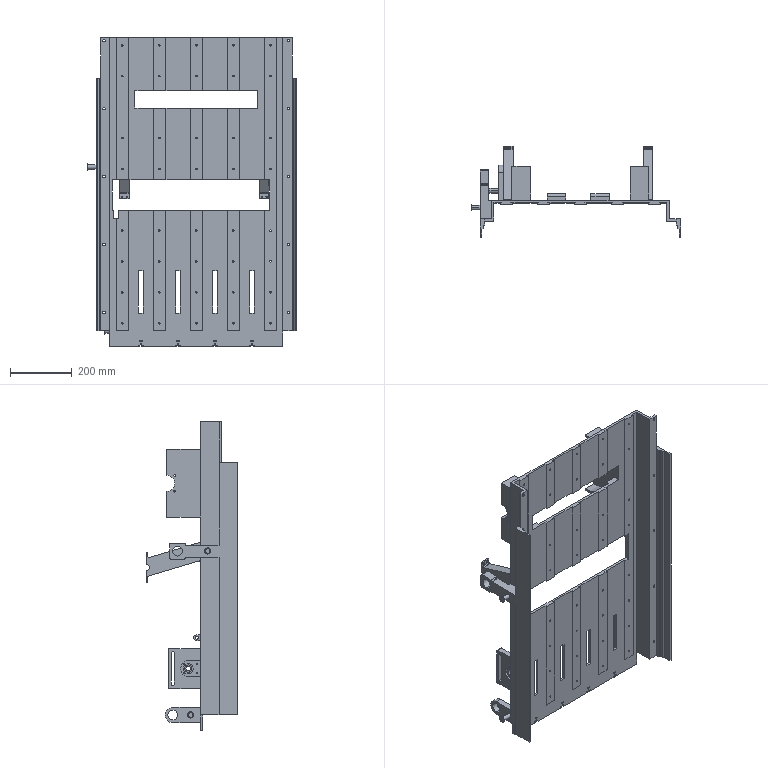Part | SolidWorks | features BaseBody 1 | 1 solid | 474 faces | box 678.27 x 295.879 x 1000 mm | volume 9669441 mm3 | cylinder 256 | plane 218 | commonest cylinder face diameters 5 x104 8 x44 3 x32 10 x24 20 x12 4 x8